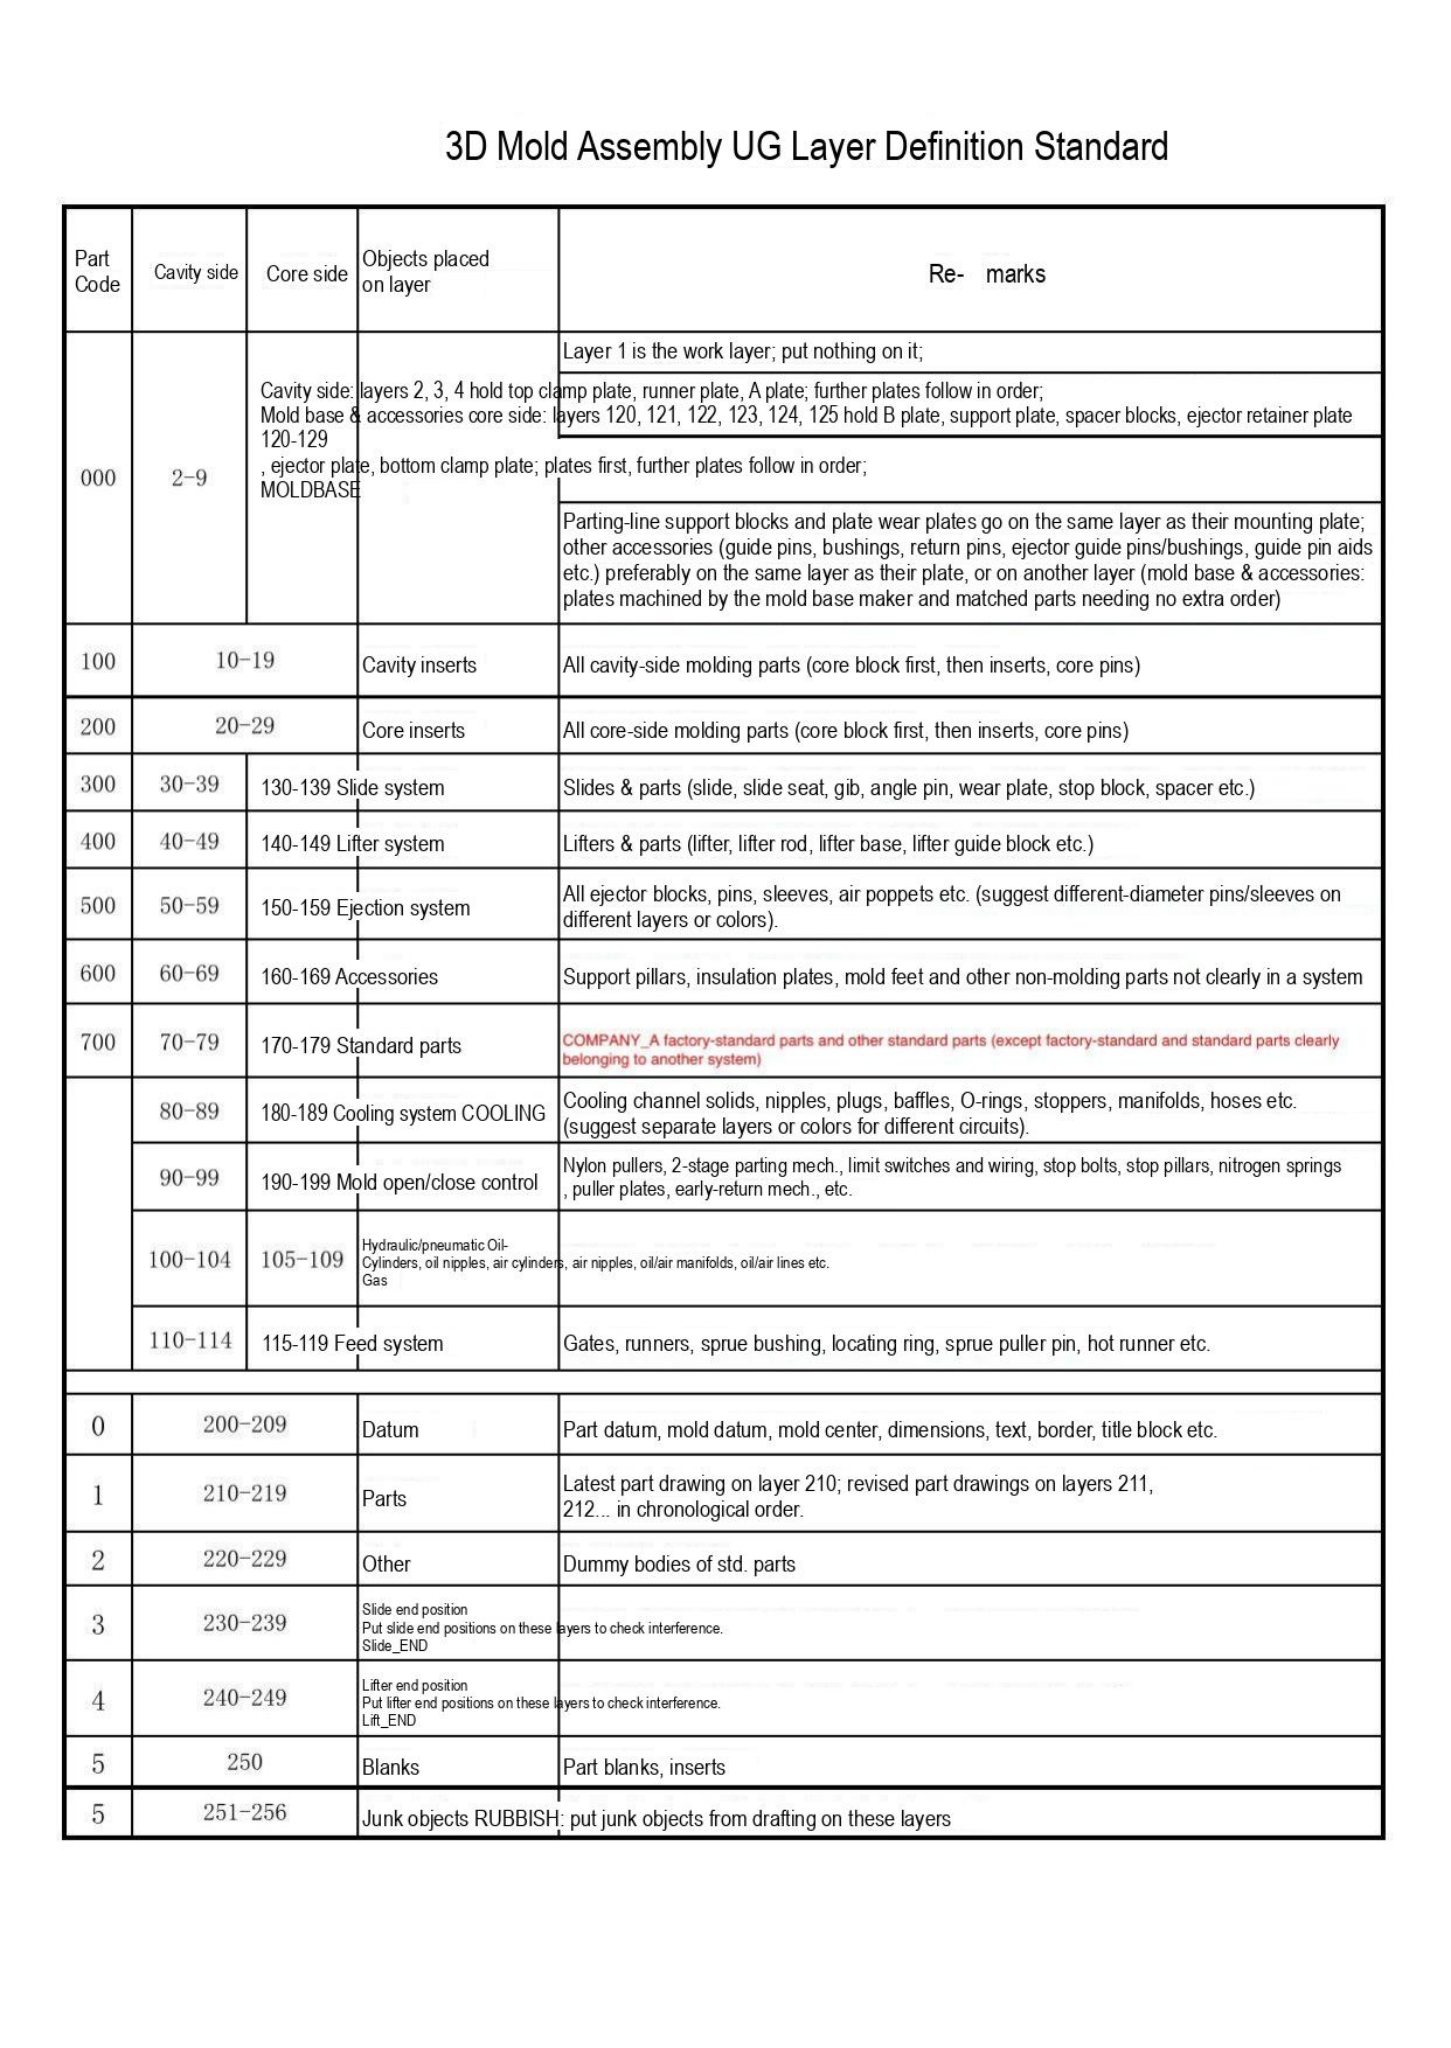# 3D Mold Assembly UG Layer Definition Standard

| Part Code | Cavity side | Core side | Objects placed on layer | Re- marks |
|---|---|---|---|---|
| 000 | 2-9 | Cavity side: layers 2, 3, 4 hold top clamp plate, runner plate, A plate; further plates follow in order; Mold base & accessories core side: layers 120, 121, 122, 123, 124, 125 hold B plate, support plate, spacer blocks, ejector retainer plate 120-129 , ejector plate, bottom clamp plate; plates first, further plates follow in order; MOLDBASE | | Layer 1 is the work layer; put nothing on it; Parting-line support blocks and plate wear plates go on the same layer as their mounting plate; other accessories (guide pins, bushings, return pins, ejector guide pins/bushings, guide pin aids etc.) preferably on the same layer as their plate, or on another layer (mold base & accessories: plates machined by the mold base maker and matched parts needing no extra order) |
| 100 | 10-19 | | Cavity inserts | All cavity-side molding parts (core block first, then inserts, core pins) |
| 200 | 20-29 | | Core inserts | All core-side molding parts (core block first, then inserts, core pins) |
| 300 | 30-39 | 130-139 | Slide system | Slides & parts (slide, slide seat, gib, angle pin, wear plate, stop block, spacer etc.) |
| 400 | 40-49 | 140-149 | Lifter system | Lifters & parts (lifter, lifter rod, lifter base, lifter guide block etc.) |
| 500 | 50-59 | 150-159 | Ejection system | All ejector blocks, pins, sleeves, air poppets etc. (suggest different-diameter pins/sleeves on different layers or colors). |
| 600 | 60-69 | 160-169 | Accessories | Support pillars, insulation plates, mold feet and other non-molding parts not clearly in a system |
| 700 | 70-79 | 170-179 | Standard parts | COMPANY_A factory-standard parts and other standard parts (except factory-standard and standard parts clearly belonging to another system) |
| | 80-89 | 180-189 | Cooling system COOLING | Cooling channel solids, nipples, plugs, baffles, O-rings, stoppers, manifolds, hoses etc. (suggest separate layers or colors for different circuits). |
| | 90-99 | 190-199 | Mold open/close control | Nylon pullers, 2-stage parting mech., limit switches and wiring, stop bolts, stop pillars, nitrogen springs , puller plates, early-return mech., etc. |
| | 100-104 | 105-109 | Hydraulic/pneumatic Oil-Gas | Cylinders, oil nipples, air cylinders, air nipples, oil/air manifolds, oil/air lines etc. |
| | 110-114 | 115-119 | Feed system | Gates, runners, sprue bushing, locating ring, sprue puller pin, hot runner etc. |
| | | | | |
| 0 | 200-209 | | Datum | Part datum, mold datum, mold center, dimensions, text, border, title block etc. |
| 1 | 210-219 | | Parts | Latest part drawing on layer 210; revised part drawings on layers 211, 212... in chronological order. |
| 2 | 220-229 | | Other | Dummy bodies of std. parts |
| 3 | 230-239 | | Slide end position Slide_END | Put slide end positions on these layers to check interference. |
| 4 | 240-249 | | Lifter end position Lift_END | Put lifter end positions on these layers to check interference. |
| 5 | 250 | | Blanks | Part blanks, inserts |
| 5 | 251-256 | | Junk objects RUBBISH | put junk objects from drafting on these layers |